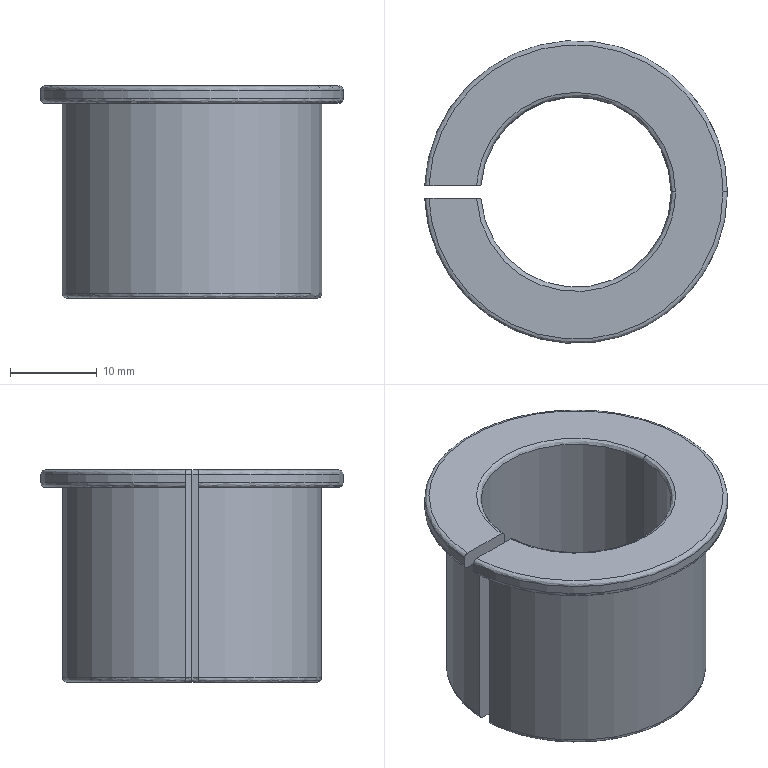Part | SolidWorks | features BaseBody 1 | 1 solid | 19 faces | box 34.984 x 35 x 24.5 mm | volume 8341 mm3 | spline 10 | plane 5 | cylinder 4 | commonest cylinder face diameters 22 x2 30 x1 35 x1